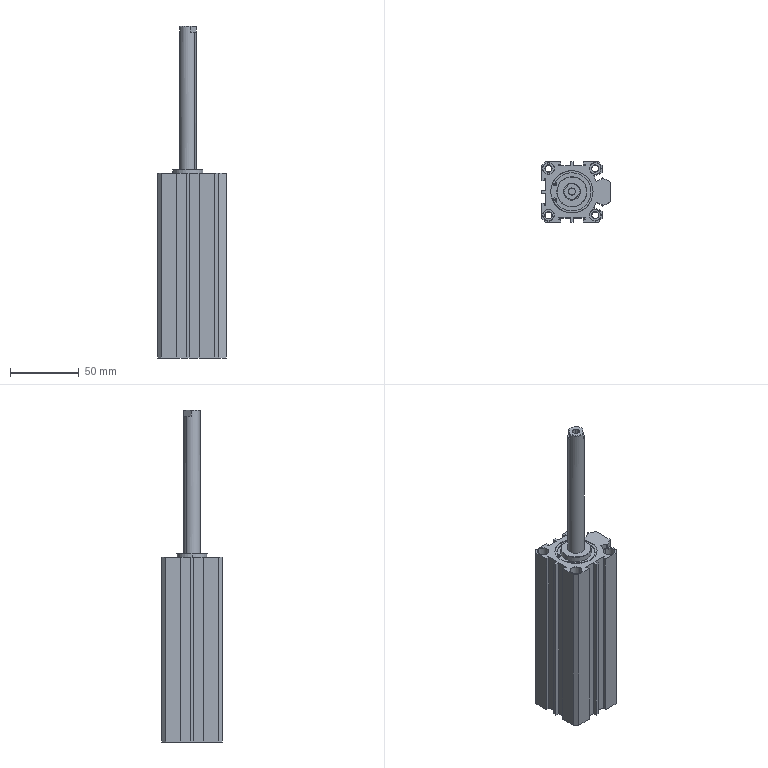Part | SolidWorks | features BaseBody 2, MoveCopyBody 1 | 2 solids | 224 faces | box 50 x 44 x 241.5 mm | volume 235412 mm3 | plane 120 | cylinder 60 | cone 40 | torus 4 | commonest cylinder face diameters 8.2 x16 2.933 x6 4.917 x6 0.978 x4 4.918 x4 8.766 x4